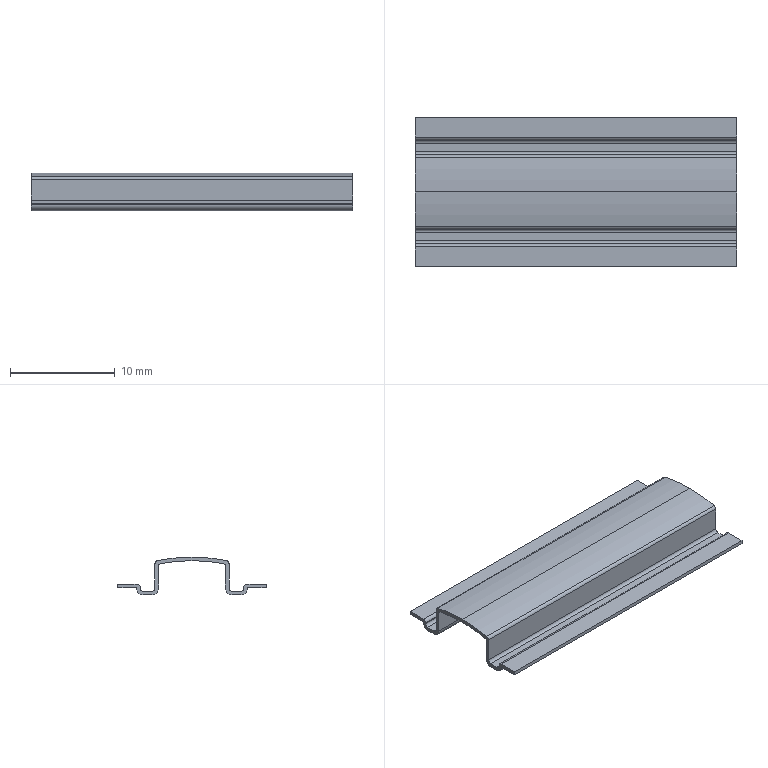Part | SolidWorks | features BaseBody 1 | 1 solid | 36 faces | box 30.643 x 14.143 x 3.615 mm | volume 220.482 mm3 | plane 20 | cylinder 16 | commonest cylinder face diameters 0.589 x8 1.296 x4 31.114 x2 31.821 x2
STEP:
#1=CARTESIAN_POINT('',(-15.321,5.304,12.964));
#2=VERTEX_POINT('',#1);
#3=CARTESIAN_POINT('',(-15.321,7.071,12.964));
#4=VERTEX_POINT('',#3);
#5=CARTESIAN_POINT('',(-15.321,5.245,12.964));
#6=DIRECTION('',(0.,1.,0.));
#7=VECTOR('',#6,1000.);
#8=LINE('',#5,#7);
#9=EDGE_CURVE('',#2,#4,#8,.T.);
#10=ORIENTED_EDGE('',*,*,#9,.F.);
#11=CARTESIAN_POINT('',(-15.321,5.304,12.944));
#12=VERTEX_POINT('',#11);
#13=CARTESIAN_POINT('',(-15.321,5.304,12.944));
#14=DIRECTION('',(0.,0.,1.));
#15=VECTOR('',#14,1000.);
#16=LINE('',#13,#15);
#17=EDGE_CURVE('',#12,#2,#16,.T.);
#18=ORIENTED_EDGE('',*,*,#17,.F.);
#19=CARTESIAN_POINT('',(-15.321,4.655,12.296));
#20=VERTEX_POINT('',#19);
#21=CARTESIAN_POINT('',(-15.321,4.655,12.944));
#22=DIRECTION('',(1.,0.,0.));
#23=DIRECTION('',(0.,0.,-1.));
#24=AXIS2_PLACEMENT_3D('',#21,#22,#23);
#25=CIRCLE('',#24,0.6482);
#26=EDGE_CURVE('',#20,#12,#25,.T.);
#27=ORIENTED_EDGE('',*,*,#26,.F.);
#28=CARTESIAN_POINT('',(-15.321,3.83,12.296));
#29=VERTEX_POINT('',#28);
#30=CARTESIAN_POINT('',(-15.321,3.83,12.296));
#31=DIRECTION('',(0.,1.,0.));
#32=VECTOR('',#31,1000.);
#33=LINE('',#30,#32);
#34=EDGE_CURVE('',#29,#20,#33,.T.);
#35=ORIENTED_EDGE('',*,*,#34,.F.);
#36=CARTESIAN_POINT('',(-15.321,3.182,12.944));
#37=VERTEX_POINT('',#36);
#38=CARTESIAN_POINT('',(-15.321,3.83,12.944));
#39=DIRECTION('',(1.,0.,0.));
#40=DIRECTION('',(0.,0.,-1.));
#41=AXIS2_PLACEMENT_3D('',#38,#39,#40);
#42=CIRCLE('',#41,0.6482);
#43=EDGE_CURVE('',#37,#29,#42,.T.);
#44=ORIENTED_EDGE('',*,*,#43,.F.);
#45=CARTESIAN_POINT('',(-15.321,3.182,15.228));
#46=VERTEX_POINT('',#45);
#47=CARTESIAN_POINT('',(-15.321,3.182,15.276));
#48=DIRECTION('',(0.,0.,-1.));
#49=VECTOR('',#48,1000.);
#50=LINE('',#47,#49);
#51=EDGE_CURVE('',#46,#37,#50,.T.);
#52=ORIENTED_EDGE('',*,*,#51,.F.);
#53=CARTESIAN_POINT('',(-15.321,0.,15.557));
#54=VERTEX_POINT('',#53);
#55=CARTESIAN_POINT('',(-15.321,0.,0.));
#56=DIRECTION('',(-1.,0.,0.));
#57=DIRECTION('',(0.,0.,-1.));
#58=AXIS2_PLACEMENT_3D('',#55,#56,#57);
#59=CIRCLE('',#58,15.557);
#60=EDGE_CURVE('',#54,#46,#59,.T.);
#61=ORIENTED_EDGE('',*,*,#60,.F.);
#62=CARTESIAN_POINT('',(-15.321,-3.182,15.228));
#63=VERTEX_POINT('',#62);
#64=CARTESIAN_POINT('',(-15.321,0.,0.));
#65=DIRECTION('',(-1.,0.,0.));
#66=DIRECTION('',(0.,0.,-1.));
#67=AXIS2_PLACEMENT_3D('',#64,#65,#66);
#68=CIRCLE('',#67,15.557);
#69=EDGE_CURVE('',#63,#54,#68,.T.);
#70=ORIENTED_EDGE('',*,*,#69,.F.);
#71=CARTESIAN_POINT('',(-15.321,-3.182,12.944));
#72=VERTEX_POINT('',#71);
#73=CARTESIAN_POINT('',(-15.321,-3.182,15.276));
#74=DIRECTION('',(0.,0.,1.));
#75=VECTOR('',#74,1000.);
#76=LINE('',#73,#75);
#77=EDGE_CURVE('',#72,#63,#76,.T.);
#78=ORIENTED_EDGE('',*,*,#77,.F.);
#79=CARTESIAN_POINT('',(-15.321,-3.83,12.296));
#80=VERTEX_POINT('',#79);
#81=CARTESIAN_POINT('',(-15.321,-3.83,12.944));
#82=DIRECTION('',(1.,0.,0.));
#83=DIRECTION('',(0.,0.,-1.));
#84=AXIS2_PLACEMENT_3D('',#81,#82,#83);
#85=CIRCLE('',#84,0.6482);
#86=EDGE_CURVE('',#80,#72,#85,.T.);
#87=ORIENTED_EDGE('',*,*,#86,.F.);
#88=CARTESIAN_POINT('',(-15.321,-4.655,12.296));
#89=VERTEX_POINT('',#88);
#90=CARTESIAN_POINT('',(-15.321,-3.83,12.296));
#91=DIRECTION('',(0.,1.,0.));
#92=VECTOR('',#91,1000.);
#93=LINE('',#90,#92);
#94=EDGE_CURVE('',#89,#80,#93,.T.);
#95=ORIENTED_EDGE('',*,*,#94,.F.);
#96=CARTESIAN_POINT('',(-15.321,-5.304,12.944));
#97=VERTEX_POINT('',#96);
#98=CARTESIAN_POINT('',(-15.321,-4.655,12.944));
#99=DIRECTION('',(1.,0.,0.));
#100=DIRECTION('',(0.,0.,-1.));
#101=AXIS2_PLACEMENT_3D('',#98,#99,#100);
#102=CIRCLE('',#101,0.6482);
#103=EDGE_CURVE('',#97,#89,#102,.T.);
#104=ORIENTED_EDGE('',*,*,#103,.F.);
#105=CARTESIAN_POINT('',(-15.321,-5.304,12.964));
#106=VERTEX_POINT('',#105);
#107=CARTESIAN_POINT('',(-15.321,-5.304,12.944));
#108=DIRECTION('',(0.,0.,-1.));
#109=VECTOR('',#108,1000.);
#110=LINE('',#107,#109);
#111=EDGE_CURVE('',#106,#97,#110,.T.);
#112=ORIENTED_EDGE('',*,*,#111,.F.);
#113=CARTESIAN_POINT('',(-15.321,-7.071,12.964));
#114=VERTEX_POINT('',#113);
#115=CARTESIAN_POINT('',(-15.321,-5.245,12.964));
#116=DIRECTION('',(0.,1.,0.));
#117=VECTOR('',#116,1000.);
#118=LINE('',#115,#117);
#119=EDGE_CURVE('',#114,#106,#118,.T.);
#120=ORIENTED_EDGE('',*,*,#119,.F.);
#121=CARTESIAN_POINT('',(-15.321,-7.071,13.318));
#122=VERTEX_POINT('',#121);
#123=CARTESIAN_POINT('',(-15.321,-7.071,12.964));
#124=DIRECTION('',(0.,0.,1.));
#125=VECTOR('',#124,1000.);
#126=LINE('',#123,#125);
#127=EDGE_CURVE('',#114,#122,#126,.T.);
#128=ORIENTED_EDGE('',*,*,#127,.T.);
#129=CARTESIAN_POINT('',(-15.321,-5.245,13.318));
#130=VERTEX_POINT('',#129);
#131=CARTESIAN_POINT('',(-15.321,-5.245,13.318));
#132=DIRECTION('',(0.,1.,0.));
#133=VECTOR('',#132,1000.);
#134=LINE('',#131,#133);
#135=EDGE_CURVE('',#122,#130,#134,.T.);
#136=ORIENTED_EDGE('',*,*,#135,.T.);
#137=CARTESIAN_POINT('',(-15.321,-4.95,13.023));
#138=VERTEX_POINT('',#137);
#139=CARTESIAN_POINT('',(-15.321,-5.245,13.023));
#140=DIRECTION('',(-1.,0.,0.));
#141=DIRECTION('',(0.,0.,1.));
#142=AXIS2_PLACEMENT_3D('',#139,#140,#141);
#143=CIRCLE('',#142,0.2946);
#144=EDGE_CURVE('',#130,#138,#143,.T.);
#145=ORIENTED_EDGE('',*,*,#144,.T.);
#146=CARTESIAN_POINT('',(-15.321,-4.95,12.944));
#147=VERTEX_POINT('',#146);
#148=CARTESIAN_POINT('',(-15.321,-4.95,12.944));
#149=DIRECTION('',(0.,0.,-1.));
#150=VECTOR('',#149,1000.);
#151=LINE('',#148,#150);
#152=EDGE_CURVE('',#138,#147,#151,.T.);
#153=ORIENTED_EDGE('',*,*,#152,.T.);
#154=CARTESIAN_POINT('',(-15.321,-4.655,12.65));
#155=VERTEX_POINT('',#154);
#156=CARTESIAN_POINT('',(-15.321,-4.655,12.944));
#157=DIRECTION('',(1.,0.,0.));
#158=DIRECTION('',(0.,0.,-1.));
#159=AXIS2_PLACEMENT_3D('',#156,#157,#158);
#160=CIRCLE('',#159,0.2946);
#161=EDGE_CURVE('',#147,#155,#160,.T.);
#162=ORIENTED_EDGE('',*,*,#161,.T.);
#163=CARTESIAN_POINT('',(-15.321,-3.83,12.65));
#164=VERTEX_POINT('',#163);
#165=CARTESIAN_POINT('',(-15.321,-3.83,12.65));
#166=DIRECTION('',(0.,1.,0.));
#167=VECTOR('',#166,1000.);
#168=LINE('',#165,#167);
#169=EDGE_CURVE('',#155,#164,#168,.T.);
#170=ORIENTED_EDGE('',*,*,#169,.T.);
#171=CARTESIAN_POINT('',(-15.321,-3.536,12.944));
#172=VERTEX_POINT('',#171);
#173=CARTESIAN_POINT('',(-15.321,-3.83,12.944));
#174=DIRECTION('',(1.,0.,0.));
#175=DIRECTION('',(0.,0.,-1.));
#176=AXIS2_PLACEMENT_3D('',#173,#174,#175);
#177=CIRCLE('',#176,0.2946);
#178=EDGE_CURVE('',#164,#172,#177,.T.);
#179=ORIENTED_EDGE('',*,*,#178,.T.);
#180=CARTESIAN_POINT('',(-15.321,-3.536,15.276));
#181=VERTEX_POINT('',#180);
#182=CARTESIAN_POINT('',(-15.321,-3.536,15.276));
#183=DIRECTION('',(0.,0.,1.));
#184=VECTOR('',#183,1000.);
#185=LINE('',#182,#184);
#186=EDGE_CURVE('',#172,#181,#185,.T.);
#187=ORIENTED_EDGE('',*,*,#186,.T.);
#188=CARTESIAN_POINT('',(-15.321,-3.302,15.564));
#189=VERTEX_POINT('',#188);
#190=CARTESIAN_POINT('',(-15.321,-3.241,15.276));
#191=DIRECTION('',(-1.,0.,0.));
#192=DIRECTION('',(0.,0.,1.));
#193=AXIS2_PLACEMENT_3D('',#190,#191,#192);
#194=CIRCLE('',#193,0.2946);
#195=EDGE_CURVE('',#181,#189,#194,.T.);
#196=ORIENTED_EDGE('',*,*,#195,.T.);
#197=CARTESIAN_POINT('',(-15.321,0.,15.911));
#198=VERTEX_POINT('',#197);
#199=CARTESIAN_POINT('',(-15.321,0.,0.));
#200=DIRECTION('',(-1.,0.,0.));
#201=DIRECTION('',(0.,0.,-1.));
#202=AXIS2_PLACEMENT_3D('',#199,#200,#201);
#203=CIRCLE('',#202,15.911);
#204=EDGE_CURVE('',#189,#198,#203,.T.);
#205=ORIENTED_EDGE('',*,*,#204,.T.);
#206=CARTESIAN_POINT('',(-15.321,3.302,15.564));
#207=VERTEX_POINT('',#206);
#208=CARTESIAN_POINT('',(-15.321,0.,0.));
#209=DIRECTION('',(-1.,0.,0.));
#210=DIRECTION('',(0.,0.,-1.));
#211=AXIS2_PLACEMENT_3D('',#208,#209,#210);
#212=CIRCLE('',#211,15.911);
#213=EDGE_CURVE('',#198,#207,#212,.T.);
#214=ORIENTED_EDGE('',*,*,#213,.T.);
#215=CARTESIAN_POINT('',(-15.321,3.536,15.276));
#216=VERTEX_POINT('',#215);
#217=CARTESIAN_POINT('',(-15.321,3.241,15.276));
#218=DIRECTION('',(-1.,0.,0.));
#219=DIRECTION('',(0.,0.,1.));
#220=AXIS2_PLACEMENT_3D('',#217,#218,#219);
#221=CIRCLE('',#220,0.2946);
#222=EDGE_CURVE('',#207,#216,#221,.T.);
#223=ORIENTED_EDGE('',*,*,#222,.T.);
#224=CARTESIAN_POINT('',(-15.321,3.536,12.944));
#225=VERTEX_POINT('',#224);
#226=CARTESIAN_POINT('',(-15.321,3.536,15.276));
#227=DIRECTION('',(0.,0.,-1.));
#228=VECTOR('',#227,1000.);
#229=LINE('',#226,#228);
#230=EDGE_CURVE('',#216,#225,#229,.T.);
#231=ORIENTED_EDGE('',*,*,#230,.T.);
#232=CARTESIAN_POINT('',(-15.321,3.83,12.65));
#233=VERTEX_POINT('',#232);
#234=CARTESIAN_POINT('',(-15.321,3.83,12.944));
#235=DIRECTION('',(1.,0.,0.));
#236=DIRECTION('',(0.,0.,-1.));
#237=AXIS2_PLACEMENT_3D('',#234,#235,#236);
#238=CIRCLE('',#237,0.2946);
#239=EDGE_CURVE('',#225,#233,#238,.T.);
#240=ORIENTED_EDGE('',*,*,#239,.T.);
#241=CARTESIAN_POINT('',(-15.321,4.655,12.65));
#242=VERTEX_POINT('',#241);
#243=CARTESIAN_POINT('',(-15.321,3.83,12.65));
#244=DIRECTION('',(0.,1.,0.));
#245=VECTOR('',#244,1000.);
#246=LINE('',#243,#245);
#247=EDGE_CURVE('',#233,#242,#246,.T.);
#248=ORIENTED_EDGE('',*,*,#247,.T.);
#249=CARTESIAN_POINT('',(-15.321,4.95,12.944));
#250=VERTEX_POINT('',#249);
#251=CARTESIAN_POINT('',(-15.321,4.655,12.944));
#252=DIRECTION('',(1.,0.,0.));
#253=DIRECTION('',(0.,0.,-1.));
#254=AXIS2_PLACEMENT_3D('',#251,#252,#253);
#255=CIRCLE('',#254,0.2946);
#256=EDGE_CURVE('',#242,#250,#255,.T.);
#257=ORIENTED_EDGE('',*,*,#256,.T.);
#258=CARTESIAN_POINT('',(-15.321,4.95,13.023));
#259=VERTEX_POINT('',#258);
#260=CARTESIAN_POINT('',(-15.321,4.95,12.944));
#261=DIRECTION('',(0.,0.,1.));
#262=VECTOR('',#261,1000.);
#263=LINE('',#260,#262);
#264=EDGE_CURVE('',#250,#259,#263,.T.);
#265=ORIENTED_EDGE('',*,*,#264,.T.);
#266=CARTESIAN_POINT('',(-15.321,5.245,13.318));
#267=VERTEX_POINT('',#266);
#268=CARTESIAN_POINT('',(-15.321,5.245,13.023));
#269=DIRECTION('',(-1.,0.,0.));
#270=DIRECTION('',(0.,0.,1.));
#271=AXIS2_PLACEMENT_3D('',#268,#269,#270);
#272=CIRCLE('',#271,0.2946);
#273=EDGE_CURVE('',#259,#267,#272,.T.);
#274=ORIENTED_EDGE('',*,*,#273,.T.);
#275=CARTESIAN_POINT('',(-15.321,7.071,13.318));
#276=VERTEX_POINT('',#275);
#277=CARTESIAN_POINT('',(-15.321,5.245,13.318));
#278=DIRECTION('',(0.,1.,0.));
#279=VECTOR('',#278,1000.);
#280=LINE('',#277,#279);
#281=EDGE_CURVE('',#267,#276,#280,.T.);
#282=ORIENTED_EDGE('',*,*,#281,.T.);
#283=CARTESIAN_POINT('',(-15.321,7.071,13.318));
#284=DIRECTION('',(0.,0.,-1.));
#285=VECTOR('',#284,1000.);
#286=LINE('',#283,#285);
#287=EDGE_CURVE('',#276,#4,#286,.T.);
#288=ORIENTED_EDGE('',*,*,#287,.T.);
#289=EDGE_LOOP('',(#10,#18,#27,#35,#44,#52,#61,#70,#78,#87,#95,#104,#112,#120,#128,#136,#145,#153,#162,#170,#179,#187,#196,#205,#214,#223,#231,#240,#248,#257,#265,#274,#282,#288));
#290=FACE_OUTER_BOUND('',#289,.T.);
#291=CARTESIAN_POINT('',(-15.321,5.245,13.023));
#292=DIRECTION('',(-1.,0.,0.));
#293=DIRECTION('',(0.,0.,1.));
#294=AXIS2_PLACEMENT_3D('',#291,#292,#293);
#295=PLANE('',#294);
#296=ADVANCED_FACE('',(#290),#295,.T.);
#297=CARTESIAN_POINT('',(15.321,5.304,12.964));
#298=VERTEX_POINT('',#297);
#299=CARTESIAN_POINT('',(15.321,7.071,12.964));
#300=VERTEX_POINT('',#299);
#301=CARTESIAN_POINT('',(15.321,5.245,12.964));
#302=DIRECTION('',(0.,1.,0.));
#303=VECTOR('',#302,1000.);
#304=LINE('',#301,#303);
#305=EDGE_CURVE('',#298,#300,#304,.T.);
#306=ORIENTED_EDGE('',*,*,#305,.T.);
#307=CARTESIAN_POINT('',(15.321,7.071,13.318));
#308=VERTEX_POINT('',#307);
#309=CARTESIAN_POINT('',(15.321,7.071,13.318));
#310=DIRECTION('',(0.,0.,-1.));
#311=VECTOR('',#310,1000.);
#312=LINE('',#309,#311);
#313=EDGE_CURVE('',#308,#300,#312,.T.);
#314=ORIENTED_EDGE('',*,*,#313,.F.);
#315=CARTESIAN_POINT('',(15.321,5.245,13.318));
#316=VERTEX_POINT('',#315);
#317=CARTESIAN_POINT('',(15.321,5.245,13.318));
#318=DIRECTION('',(0.,1.,0.));
#319=VECTOR('',#318,1000.);
#320=LINE('',#317,#319);
#321=EDGE_CURVE('',#316,#308,#320,.T.);
#322=ORIENTED_EDGE('',*,*,#321,.F.);
#323=CARTESIAN_POINT('',(15.321,4.95,13.023));
#324=VERTEX_POINT('',#323);
#325=CARTESIAN_POINT('',(15.321,5.245,13.023));
#326=DIRECTION('',(-1.,0.,0.));
#327=DIRECTION('',(0.,0.,1.));
#328=AXIS2_PLACEMENT_3D('',#325,#326,#327);
#329=CIRCLE('',#328,0.2946);
#330=EDGE_CURVE('',#324,#316,#329,.T.);
#331=ORIENTED_EDGE('',*,*,#330,.F.);
#332=CARTESIAN_POINT('',(15.321,4.95,12.944));
#333=VERTEX_POINT('',#332);
#334=CARTESIAN_POINT('',(15.321,4.95,12.944));
#335=DIRECTION('',(0.,0.,1.));
#336=VECTOR('',#335,1000.);
#337=LINE('',#334,#336);
#338=EDGE_CURVE('',#333,#324,#337,.T.);
#339=ORIENTED_EDGE('',*,*,#338,.F.);
#340=CARTESIAN_POINT('',(15.321,4.655,12.65));
#341=VERTEX_POINT('',#340);
#342=CARTESIAN_POINT('',(15.321,4.655,12.944));
#343=DIRECTION('',(1.,0.,0.));
#344=DIRECTION('',(0.,0.,-1.));
#345=AXIS2_PLACEMENT_3D('',#342,#343,#344);
#346=CIRCLE('',#345,0.2946);
#347=EDGE_CURVE('',#341,#333,#346,.T.);
#348=ORIENTED_EDGE('',*,*,#347,.F.);
#349=CARTESIAN_POINT('',(15.321,3.83,12.65));
#350=VERTEX_POINT('',#349);
#351=CARTESIAN_POINT('',(15.321,3.83,12.65));
#352=DIRECTION('',(0.,1.,0.));
#353=VECTOR('',#352,1000.);
#354=LINE('',#351,#353);
#355=EDGE_CURVE('',#350,#341,#354,.T.);
#356=ORIENTED_EDGE('',*,*,#355,.F.);
#357=CARTESIAN_POINT('',(15.321,3.536,12.944));
#358=VERTEX_POINT('',#357);
#359=CARTESIAN_POINT('',(15.321,3.83,12.944));
#360=DIRECTION('',(1.,0.,0.));
#361=DIRECTION('',(0.,0.,-1.));
#362=AXIS2_PLACEMENT_3D('',#359,#360,#361);
#363=CIRCLE('',#362,0.2946);
#364=EDGE_CURVE('',#358,#350,#363,.T.);
#365=ORIENTED_EDGE('',*,*,#364,.F.);
#366=CARTESIAN_POINT('',(15.321,3.536,15.276));
#367=VERTEX_POINT('',#366);
#368=CARTESIAN_POINT('',(15.321,3.536,15.276));
#369=DIRECTION('',(0.,0.,-1.));
#370=VECTOR('',#369,1000.);
#371=LINE('',#368,#370);
#372=EDGE_CURVE('',#367,#358,#371,.T.);
#373=ORIENTED_EDGE('',*,*,#372,.F.);
#374=CARTESIAN_POINT('',(15.321,3.302,15.564));
#375=VERTEX_POINT('',#374);
#376=CARTESIAN_POINT('',(15.321,3.241,15.276));
#377=DIRECTION('',(-1.,0.,0.));
#378=DIRECTION('',(0.,0.,1.));
#379=AXIS2_PLACEMENT_3D('',#376,#377,#378);
#380=CIRCLE('',#379,0.2946);
#381=EDGE_CURVE('',#375,#367,#380,.T.);
#382=ORIENTED_EDGE('',*,*,#381,.F.);
#383=CARTESIAN_POINT('',(15.321,0.,15.911));
#384=VERTEX_POINT('',#383);
#385=CARTESIAN_POINT('',(15.321,0.,0.));
#386=DIRECTION('',(-1.,0.,0.));
#387=DIRECTION('',(0.,0.,-1.));
#388=AXIS2_PLACEMENT_3D('',#385,#386,#387);
#389=CIRCLE('',#388,15.911);
#390=EDGE_CURVE('',#384,#375,#389,.T.);
#391=ORIENTED_EDGE('',*,*,#390,.F.);
#392=CARTESIAN_POINT('',(15.321,-3.302,15.564));
#393=VERTEX_POINT('',#392);
#394=CARTESIAN_POINT('',(15.321,0.,0.));
#395=DIRECTION('',(-1.,0.,0.));
#396=DIRECTION('',(0.,0.,-1.));
#397=AXIS2_PLACEMENT_3D('',#394,#395,#396);
#398=CIRCLE('',#397,15.911);
#399=EDGE_CURVE('',#393,#384,#398,.T.);
#400=ORIENTED_EDGE('',*,*,#399,.F.);
#401=CARTESIAN_POINT('',(15.321,-3.536,15.276));
#402=VERTEX_POINT('',#401);
#403=CARTESIAN_POINT('',(15.321,-3.241,15.276));
#404=DIRECTION('',(-1.,0.,0.));
#405=DIRECTION('',(0.,0.,1.));
#406=AXIS2_PLACEMENT_3D('',#403,#404,#405);
#407=CIRCLE('',#406,0.2946);
#408=EDGE_CURVE('',#402,#393,#407,.T.);
#409=ORIENTED_EDGE('',*,*,#408,.F.);
#410=CARTESIAN_POINT('',(15.321,-3.536,12.944));
#411=VERTEX_POINT('',#410);
#412=CARTESIAN_POINT('',(15.321,-3.536,15.276));
#413=DIRECTION('',(0.,0.,1.));
#414=VECTOR('',#413,1000.);
#415=LINE('',#412,#414);
#416=EDGE_CURVE('',#411,#402,#415,.T.);
#417=ORIENTED_EDGE('',*,*,#416,.F.);
#418=CARTESIAN_POINT('',(15.321,-3.83,12.65));
#419=VERTEX_POINT('',#418);
#420=CARTESIAN_POINT('',(15.321,-3.83,12.944));
#421=DIRECTION('',(1.,0.,0.));
#422=DIRECTION('',(0.,0.,-1.));
#423=AXIS2_PLACEMENT_3D('',#420,#421,#422);
#424=CIRCLE('',#423,0.2946);
#425=EDGE_CURVE('',#419,#411,#424,.T.);
#426=ORIENTED_EDGE('',*,*,#425,.F.);
#427=CARTESIAN_POINT('',(15.321,-4.655,12.65));
#428=VERTEX_POINT('',#427);
#429=CARTESIAN_POINT('',(15.321,-3.83,12.65));
#430=DIRECTION('',(0.,1.,0.));
#431=VECTOR('',#430,1000.);
#432=LINE('',#429,#431);
#433=EDGE_CURVE('',#428,#419,#432,.T.);
#434=ORIENTED_EDGE('',*,*,#433,.F.);
#435=CARTESIAN_POINT('',(15.321,-4.95,12.944));
#436=VERTEX_POINT('',#435);
#437=CARTESIAN_POINT('',(15.321,-4.655,12.944));
#438=DIRECTION('',(1.,0.,0.));
#439=DIRECTION('',(0.,0.,-1.));
#440=AXIS2_PLACEMENT_3D('',#437,#438,#439);
#441=CIRCLE('',#440,0.2946);
#442=EDGE_CURVE('',#436,#428,#441,.T.);
#443=ORIENTED_EDGE('',*,*,#442,.F.);
#444=CARTESIAN_POINT('',(15.321,-4.95,13.023));
#445=VERTEX_POINT('',#444);
#446=CARTESIAN_POINT('',(15.321,-4.95,12.944));
#447=DIRECTION('',(0.,0.,-1.));
#448=VECTOR('',#447,1000.);
#449=LINE('',#446,#448);
#450=EDGE_CURVE('',#445,#436,#449,.T.);
#451=ORIENTED_EDGE('',*,*,#450,.F.);
#452=CARTESIAN_POINT('',(15.321,-5.245,13.318));
#453=VERTEX_POINT('',#452);
#454=CARTESIAN_POINT('',(15.321,-5.245,13.023));
#455=DIRECTION('',(-1.,0.,0.));
#456=DIRECTION('',(0.,0.,1.));
#457=AXIS2_PLACEMENT_3D('',#454,#455,#456);
#458=CIRCLE('',#457,0.2946);
#459=EDGE_CURVE('',#453,#445,#458,.T.);
#460=ORIENTED_EDGE('',*,*,#459,.F.);
#461=CARTESIAN_POINT('',(15.321,-7.071,13.318));
#462=VERTEX_POINT('',#461);
#463=CARTESIAN_POINT('',(15.321,-5.245,13.318));
#464=DIRECTION('',(0.,1.,0.));
#465=VECTOR('',#464,1000.);
#466=LINE('',#463,#465);
#467=EDGE_CURVE('',#462,#453,#466,.T.);
#468=ORIENTED_EDGE('',*,*,#467,.F.);
#469=CARTESIAN_POINT('',(15.321,-7.071,12.964));
#470=VERTEX_POINT('',#469);
#471=CARTESIAN_POINT('',(15.321,-7.071,12.964));
#472=DIRECTION('',(0.,0.,1.));
#473=VECTOR('',#472,1000.);
#474=LINE('',#471,#473);
#475=EDGE_CURVE('',#470,#462,#474,.T.);
#476=ORIENTED_EDGE('',*,*,#475,.F.);
#477=CARTESIAN_POINT('',(15.321,-5.304,12.964));
#478=VERTEX_POINT('',#477);
#479=CARTESIAN_POINT('',(15.321,-5.245,12.964));
#480=DIRECTION('',(0.,1.,0.));
#481=VECTOR('',#480,1000.);
#482=LINE('',#479,#481);
#483=EDGE_CURVE('',#470,#478,#482,.T.);
#484=ORIENTED_EDGE('',*,*,#483,.T.);
#485=CARTESIAN_POINT('',(15.321,-5.304,12.944));
#486=VERTEX_POINT('',#485);
#487=CARTESIAN_POINT('',(15.321,-5.304,12.944));
#488=DIRECTION('',(0.,0.,-1.));
#489=VECTOR('',#488,1000.);
#490=LINE('',#487,#489);
#491=EDGE_CURVE('',#478,#486,#490,.T.);
#492=ORIENTED_EDGE('',*,*,#491,.T.);
#493=CARTESIAN_POINT('',(15.321,-4.655,12.296));
#494=VERTEX_POINT('',#493);
#495=CARTESIAN_POINT('',(15.321,-4.655,12.944));
#496=DIRECTION('',(1.,0.,0.));
#497=DIRECTION('',(0.,0.,-1.));
#498=AXIS2_PLACEMENT_3D('',#495,#496,#497);
#499=CIRCLE('',#498,0.6482);
#500=EDGE_CURVE('',#486,#494,#499,.T.);
#501=ORIENTED_EDGE('',*,*,#500,.T.);
#502=CARTESIAN_POINT('',(15.321,-3.83,12.296));
#503=VERTEX_POINT('',#502);
#504=CARTESIAN_POINT('',(15.321,-3.83,12.296));
#505=DIRECTION('',(0.,1.,0.));
#506=VECTOR('',#505,1000.);
#507=LINE('',#504,#506);
#508=EDGE_CURVE('',#494,#503,#507,.T.);
#509=ORIENTED_EDGE('',*,*,#508,.T.);
#510=CARTESIAN_POINT('',(15.321,-3.182,12.944));
#511=VERTEX_POINT('',#510);
#512=CARTESIAN_POINT('',(15.321,-3.83,12.944));
#513=DIRECTION('',(1.,0.,0.));
#514=DIRECTION('',(0.,0.,-1.));
#515=AXIS2_PLACEMENT_3D('',#512,#513,#514);
#516=CIRCLE('',#515,0.6482);
#517=EDGE_CURVE('',#503,#511,#516,.T.);
#518=ORIENTED_EDGE('',*,*,#517,.T.);
#519=CARTESIAN_POINT('',(15.321,-3.182,15.228));
#520=VERTEX_POINT('',#519);
#521=CARTESIAN_POINT('',(15.321,-3.182,15.276));
#522=DIRECTION('',(0.,0.,1.));
#523=VECTOR('',#522,1000.);
#524=LINE('',#521,#523);
#525=EDGE_CURVE('',#511,#520,#524,.T.);
#526=ORIENTED_EDGE('',*,*,#525,.T.);
#527=CARTESIAN_POINT('',(15.321,0.,15.557));
#528=VERTEX_POINT('',#527);
#529=CARTESIAN_POINT('',(15.321,0.,0.));
#530=DIRECTION('',(-1.,0.,0.));
#531=DIRECTION('',(0.,0.,-1.));
#532=AXIS2_PLACEMENT_3D('',#529,#530,#531);
#533=CIRCLE('',#532,15.557);
#534=EDGE_CURVE('',#520,#528,#533,.T.);
#535=ORIENTED_EDGE('',*,*,#534,.T.);
#536=CARTESIAN_POINT('',(15.321,3.182,15.228));
#537=VERTEX_POINT('',#536);
#538=CARTESIAN_POINT('',(15.321,0.,0.));
#539=DIRECTION('',(-1.,0.,0.));
#540=DIRECTION('',(0.,0.,-1.));
#541=AXIS2_PLACEMENT_3D('',#538,#539,#540);
#542=CIRCLE('',#541,15.557);
#543=EDGE_CURVE('',#528,#537,#542,.T.);
#544=ORIENTED_EDGE('',*,*,#543,.T.);
#545=CARTESIAN_POINT('',(15.321,3.182,12.944));
#546=VERTEX_POINT('',#545);
#547=CARTESIAN_POINT('',(15.321,3.182,15.276));
#548=DIRECTION('',(0.,0.,-1.));
#549=VECTOR('',#548,1000.);
#550=LINE('',#547,#549);
#551=EDGE_CURVE('',#537,#546,#550,.T.);
#552=ORIENTED_EDGE('',*,*,#551,.T.);
#553=CARTESIAN_POINT('',(15.321,3.83,12.296));
#554=VERTEX_POINT('',#553);
#555=CARTESIAN_POINT('',(15.321,3.83,12.944));
#556=DIRECTION('',(1.,0.,0.));
#557=DIRECTION('',(0.,0.,-1.));
#558=AXIS2_PLACEMENT_3D('',#555,#556,#557);
#559=CIRCLE('',#558,0.6482);
#560=EDGE_CURVE('',#546,#554,#559,.T.);
#561=ORIENTED_EDGE('',*,*,#560,.T.);
#562=CARTESIAN_POINT('',(15.321,4.655,12.296));
#563=VERTEX_POINT('',#562);
#564=CARTESIAN_POINT('',(15.321,3.83,12.296));
#565=DIRECTION('',(0.,1.,0.));
#566=VECTOR('',#565,1000.);
#567=LINE('',#564,#566);
#568=EDGE_CURVE('',#554,#563,#567,.T.);
#569=ORIENTED_EDGE('',*,*,#568,.T.);
#570=CARTESIAN_POINT('',(15.321,5.304,12.944));
#571=VERTEX_POINT('',#570);
#572=CARTESIAN_POINT('',(15.321,4.655,12.944));
#573=DIRECTION('',(1.,0.,0.));
#574=DIRECTION('',(0.,0.,-1.));
#575=AXIS2_PLACEMENT_3D('',#572,#573,#574);
#576=CIRCLE('',#575,0.6482);
#577=EDGE_CURVE('',#563,#571,#576,.T.);
#578=ORIENTED_EDGE('',*,*,#577,.T.);
#579=CARTESIAN_POINT('',(15.321,5.304,12.944));
#580=DIRECTION('',(0.,0.,1.));
#581=VECTOR('',#580,1000.);
#582=LINE('',#579,#581);
#583=EDGE_CURVE('',#571,#298,#582,.T.);
#584=ORIENTED_EDGE('',*,*,#583,.T.);
#585=EDGE_LOOP('',(#306,#314,#322,#331,#339,#348,#356,#365,#373,#382,#391,#400,#409,#417,#426,#434,#443,#451,#460,#468,#476,#484,#492,#501,#509,#518,#526,#535,#544,#552,#561,#569,#578,#584));
#586=FACE_OUTER_BOUND('',#585,.T.);
#587=CARTESIAN_POINT('',(15.321,5.245,13.023));
#588=DIRECTION('',(-1.,0.,0.));
#589=DIRECTION('',(0.,0.,1.));
#590=AXIS2_PLACEMENT_3D('',#587,#588,#589);
#591=PLANE('',#590);
#592=ADVANCED_FACE('',(#586),#591,.F.);
#593=ORIENTED_EDGE('',*,*,#17,.T.);
#594=CARTESIAN_POINT('',(15.321,5.304,12.964));
#595=DIRECTION('',(-1.,0.,0.));
#596=VECTOR('',#595,1000.);
#597=LINE('',#594,#596);
#598=EDGE_CURVE('',#298,#2,#597,.T.);
#599=ORIENTED_EDGE('',*,*,#598,.F.);
#600=ORIENTED_EDGE('',*,*,#583,.F.);
#601=CARTESIAN_POINT('',(15.321,5.304,12.944));
#602=DIRECTION('',(-1.,0.,0.));
#603=VECTOR('',#602,1000.);
#604=LINE('',#601,#603);
#605=EDGE_CURVE('',#571,#12,#604,.T.);
#606=ORIENTED_EDGE('',*,*,#605,.T.);
#607=EDGE_LOOP('',(#593,#599,#600,#606));
#608=FACE_OUTER_BOUND('',#607,.T.);
#609=CARTESIAN_POINT('',(15.321,5.304,12.944));
#610=DIRECTION('',(0.,-1.,0.));
#611=DIRECTION('',(0.,0.,-1.));
#612=AXIS2_PLACEMENT_3D('',#609,#610,#611);
#613=PLANE('',#612);
#614=ADVANCED_FACE('',(#608),#613,.F.);
#615=ORIENTED_EDGE('',*,*,#26,.T.);
#616=ORIENTED_EDGE('',*,*,#605,.F.);
#617=ORIENTED_EDGE('',*,*,#577,.F.);
#618=CARTESIAN_POINT('',(15.321,4.655,12.296));
#619=DIRECTION('',(-1.,0.,0.));
#620=VECTOR('',#619,1000.);
#621=LINE('',#618,#620);
#622=EDGE_CURVE('',#563,#20,#621,.T.);
#623=ORIENTED_EDGE('',*,*,#622,.T.);
#624=EDGE_LOOP('',(#615,#616,#617,#623));
#625=FACE_OUTER_BOUND('',#624,.T.);
#626=CARTESIAN_POINT('',(15.321,4.655,12.944));
#627=DIRECTION('',(-1.,0.,0.));
#628=DIRECTION('',(0.,0.,1.));
#629=AXIS2_PLACEMENT_3D('',#626,#627,#628);
#630=CYLINDRICAL_SURFACE('',#629,0.6482);
#631=ADVANCED_FACE('',(#625),#630,.T.);
#632=ORIENTED_EDGE('',*,*,#34,.T.);
#633=ORIENTED_EDGE('',*,*,#622,.F.);
#634=ORIENTED_EDGE('',*,*,#568,.F.);
#635=CARTESIAN_POINT('',(15.321,3.83,12.296));
#636=DIRECTION('',(-1.,0.,0.));
#637=VECTOR('',#636,1000.);
#638=LINE('',#635,#637);
#639=EDGE_CURVE('',#554,#29,#638,.T.);
#640=ORIENTED_EDGE('',*,*,#639,.T.);
#641=EDGE_LOOP('',(#632,#633,#634,#640));
#642=FACE_OUTER_BOUND('',#641,.T.);
#643=CARTESIAN_POINT('',(15.321,3.83,12.296));
#644=DIRECTION('',(0.,0.,1.));
#645=DIRECTION('',(1.,0.,0.));
#646=AXIS2_PLACEMENT_3D('',#643,#644,#645);
#647=PLANE('',#646);
#648=ADVANCED_FACE('',(#642),#647,.F.);
#649=ORIENTED_EDGE('',*,*,#43,.T.);
#650=ORIENTED_EDGE('',*,*,#639,.F.);
#651=ORIENTED_EDGE('',*,*,#560,.F.);
#652=CARTESIAN_POINT('',(15.321,3.182,12.944));
#653=DIRECTION('',(-1.,0.,0.));
#654=VECTOR('',#653,1000.);
#655=LINE('',#652,#654);
#656=EDGE_CURVE('',#546,#37,#655,.T.);
#657=ORIENTED_EDGE('',*,*,#656,.T.);
#658=EDGE_LOOP('',(#649,#650,#651,#657));
#659=FACE_OUTER_BOUND('',#658,.T.);
#660=CARTESIAN_POINT('',(15.321,3.83,12.944));
#661=DIRECTION('',(-1.,0.,0.));
#662=DIRECTION('',(0.,0.,1.));
#663=AXIS2_PLACEMENT_3D('',#660,#661,#662);
#664=CYLINDRICAL_SURFACE('',#663,0.6482);
#665=ADVANCED_FACE('',(#659),#664,.T.);
#666=ORIENTED_EDGE('',*,*,#51,.T.);
#667=ORIENTED_EDGE('',*,*,#656,.F.);
#668=ORIENTED_EDGE('',*,*,#551,.F.);
#669=CARTESIAN_POINT('',(15.321,3.182,15.228));
#670=DIRECTION('',(-1.,0.,0.));
#671=VECTOR('',#670,1000.);
#672=LINE('',#669,#671);
#673=EDGE_CURVE('',#537,#46,#672,.T.);
#674=ORIENTED_EDGE('',*,*,#673,.T.);
#675=EDGE_LOOP('',(#666,#667,#668,#674));
#676=FACE_OUTER_BOUND('',#675,.T.);
#677=CARTESIAN_POINT('',(15.321,3.182,15.276));
#678=DIRECTION('',(0.,1.,0.));
#679=DIRECTION('',(1.,0.,0.));
#680=AXIS2_PLACEMENT_3D('',#677,#678,#679);
#681=PLANE('',#680);
#682=ADVANCED_FACE('',(#676),#681,.F.);
#683=CARTESIAN_POINT('',(15.321,0.,15.557));
#684=DIRECTION('',(-1.,0.,0.));
#685=VECTOR('',#684,1000.);
#686=LINE('',#683,#685);
#687=EDGE_CURVE('',#528,#54,#686,.T.);
#688=ORIENTED_EDGE('',*,*,#687,.F.);
#689=ORIENTED_EDGE('',*,*,#534,.F.);
#690=CARTESIAN_POINT('',(15.321,-3.182,15.228));
#691=DIRECTION('',(-1.,0.,0.));
#692=VECTOR('',#691,1000.);
#693=LINE('',#690,#692);
#694=EDGE_CURVE('',#520,#63,#693,.T.);
#695=ORIENTED_EDGE('',*,*,#694,.T.);
#696=ORIENTED_EDGE('',*,*,#69,.T.);
#697=EDGE_LOOP('',(#688,#689,#695,#696));
#698=FACE_OUTER_BOUND('',#697,.T.);
#699=CARTESIAN_POINT('',(15.321,0.,0.));
#700=DIRECTION('',(-1.,0.,0.));
#701=DIRECTION('',(0.,0.,1.));
#702=AXIS2_PLACEMENT_3D('',#699,#700,#701);
#703=CYLINDRICAL_SURFACE('',#702,15.557);
#704=ADVANCED_FACE('',(#698),#703,.F.);
#705=ORIENTED_EDGE('',*,*,#77,.T.);
#706=ORIENTED_EDGE('',*,*,#694,.F.);
#707=ORIENTED_EDGE('',*,*,#525,.F.);
#708=CARTESIAN_POINT('',(15.321,-3.182,12.944));
#709=DIRECTION('',(-1.,0.,0.));
#710=VECTOR('',#709,1000.);
#711=LINE('',#708,#710);
#712=EDGE_CURVE('',#511,#72,#711,.T.);
#713=ORIENTED_EDGE('',*,*,#712,.T.);
#714=EDGE_LOOP('',(#705,#706,#707,#713));
#715=FACE_OUTER_BOUND('',#714,.T.);
#716=CARTESIAN_POINT('',(15.321,-3.182,15.276));
#717=DIRECTION('',(0.,-1.,0.));
#718=DIRECTION('',(0.,0.,-1.));
#719=AXIS2_PLACEMENT_3D('',#716,#717,#718);
#720=PLANE('',#719);
#721=ADVANCED_FACE('',(#715),#720,.F.);
#722=ORIENTED_EDGE('',*,*,#86,.T.);
#723=ORIENTED_EDGE('',*,*,#712,.F.);
#724=ORIENTED_EDGE('',*,*,#517,.F.);
#725=CARTESIAN_POINT('',(15.321,-3.83,12.296));
#726=DIRECTION('',(-1.,0.,0.));
#727=VECTOR('',#726,1000.);
#728=LINE('',#725,#727);
#729=EDGE_CURVE('',#503,#80,#728,.T.);
#730=ORIENTED_EDGE('',*,*,#729,.T.);
#731=EDGE_LOOP('',(#722,#723,#724,#730));
#732=FACE_OUTER_BOUND('',#731,.T.);
#733=CARTESIAN_POINT('',(15.321,-3.83,12.944));
#734=DIRECTION('',(-1.,0.,0.));
#735=DIRECTION('',(0.,0.,1.));
#736=AXIS2_PLACEMENT_3D('',#733,#734,#735);
#737=CYLINDRICAL_SURFACE('',#736,0.6482);
#738=ADVANCED_FACE('',(#732),#737,.T.);
#739=ORIENTED_EDGE('',*,*,#94,.T.);
#740=ORIENTED_EDGE('',*,*,#729,.F.);
#741=ORIENTED_EDGE('',*,*,#508,.F.);
#742=CARTESIAN_POINT('',(15.321,-4.655,12.296));
#743=DIRECTION('',(-1.,0.,0.));
#744=VECTOR('',#743,1000.);
#745=LINE('',#742,#744);
#746=EDGE_CURVE('',#494,#89,#745,.T.);
#747=ORIENTED_EDGE('',*,*,#746,.T.);
#748=EDGE_LOOP('',(#739,#740,#741,#747));
#749=FACE_OUTER_BOUND('',#748,.T.);
#750=CARTESIAN_POINT('',(15.321,-3.83,12.296));
#751=DIRECTION('',(0.,0.,1.));
#752=DIRECTION('',(1.,0.,0.));
#753=AXIS2_PLACEMENT_3D('',#750,#751,#752);
#754=PLANE('',#753);
#755=ADVANCED_FACE('',(#749),#754,.F.);
#756=ORIENTED_EDGE('',*,*,#103,.T.);
#757=ORIENTED_EDGE('',*,*,#746,.F.);
#758=ORIENTED_EDGE('',*,*,#500,.F.);
#759=CARTESIAN_POINT('',(15.321,-5.304,12.944));
#760=DIRECTION('',(-1.,0.,0.));
#761=VECTOR('',#760,1000.);
#762=LINE('',#759,#761);
#763=EDGE_CURVE('',#486,#97,#762,.T.);
#764=ORIENTED_EDGE('',*,*,#763,.T.);
#765=EDGE_LOOP('',(#756,#757,#758,#764));
#766=FACE_OUTER_BOUND('',#765,.T.);
#767=CARTESIAN_POINT('',(15.321,-4.655,12.944));
#768=DIRECTION('',(-1.,0.,0.));
#769=DIRECTION('',(0.,0.,1.));
#770=AXIS2_PLACEMENT_3D('',#767,#768,#769);
#771=CYLINDRICAL_SURFACE('',#770,0.6482);
#772=ADVANCED_FACE('',(#766),#771,.T.);
#773=ORIENTED_EDGE('',*,*,#111,.T.);
#774=ORIENTED_EDGE('',*,*,#763,.F.);
#775=ORIENTED_EDGE('',*,*,#491,.F.);
#776=CARTESIAN_POINT('',(15.321,-5.304,12.964));
#777=DIRECTION('',(-1.,0.,0.));
#778=VECTOR('',#777,1000.);
#779=LINE('',#776,#778);
#780=EDGE_CURVE('',#478,#106,#779,.T.);
#781=ORIENTED_EDGE('',*,*,#780,.T.);
#782=EDGE_LOOP('',(#773,#774,#775,#781));
#783=FACE_OUTER_BOUND('',#782,.T.);
#784=CARTESIAN_POINT('',(15.321,-5.304,12.944));
#785=DIRECTION('',(0.,1.,0.));
#786=DIRECTION('',(1.,0.,0.));
#787=AXIS2_PLACEMENT_3D('',#784,#785,#786);
#788=PLANE('',#787);
#789=ADVANCED_FACE('',(#783),#788,.F.);
#790=ORIENTED_EDGE('',*,*,#119,.T.);
#791=ORIENTED_EDGE('',*,*,#780,.F.);
#792=ORIENTED_EDGE('',*,*,#483,.F.);
#793=CARTESIAN_POINT('',(15.321,-7.071,12.964));
#794=DIRECTION('',(-1.,0.,0.));
#795=VECTOR('',#794,1000.);
#796=LINE('',#793,#795);
#797=EDGE_CURVE('',#470,#114,#796,.T.);
#798=ORIENTED_EDGE('',*,*,#797,.T.);
#799=EDGE_LOOP('',(#790,#791,#792,#798));
#800=FACE_OUTER_BOUND('',#799,.T.);
#801=CARTESIAN_POINT('',(15.321,-5.245,12.964));
#802=DIRECTION('',(0.,0.,1.));
#803=DIRECTION('',(1.,0.,0.));
#804=AXIS2_PLACEMENT_3D('',#801,#802,#803);
#805=PLANE('',#804);
#806=ADVANCED_FACE('',(#800),#805,.F.);
#807=ORIENTED_EDGE('',*,*,#127,.F.);
#808=ORIENTED_EDGE('',*,*,#797,.F.);
#809=ORIENTED_EDGE('',*,*,#475,.T.);
#810=CARTESIAN_POINT('',(15.321,-7.071,13.318));
#811=DIRECTION('',(-1.,0.,0.));
#812=VECTOR('',#811,1000.);
#813=LINE('',#810,#812);
#814=EDGE_CURVE('',#462,#122,#813,.T.);
#815=ORIENTED_EDGE('',*,*,#814,.T.);
#816=EDGE_LOOP('',(#807,#808,#809,#815));
#817=FACE_OUTER_BOUND('',#816,.T.);
#818=CARTESIAN_POINT('',(15.321,-7.071,12.964));
#819=DIRECTION('',(0.,-1.,0.));
#820=DIRECTION('',(0.,0.,-1.));
#821=AXIS2_PLACEMENT_3D('',#818,#819,#820);
#822=PLANE('',#821);
#823=ADVANCED_FACE('',(#817),#822,.T.);
#824=ORIENTED_EDGE('',*,*,#135,.F.);
#825=ORIENTED_EDGE('',*,*,#814,.F.);
#826=ORIENTED_EDGE('',*,*,#467,.T.);
#827=CARTESIAN_POINT('',(15.321,-5.245,13.318));
#828=DIRECTION('',(-1.,0.,0.));
#829=VECTOR('',#828,1000.);
#830=LINE('',#827,#829);
#831=EDGE_CURVE('',#453,#130,#830,.T.);
#832=ORIENTED_EDGE('',*,*,#831,.T.);
#833=EDGE_LOOP('',(#824,#825,#826,#832));
#834=FACE_OUTER_BOUND('',#833,.T.);
#835=CARTESIAN_POINT('',(15.321,-5.245,13.318));
#836=DIRECTION('',(0.,0.,1.));
#837=DIRECTION('',(1.,0.,0.));
#838=AXIS2_PLACEMENT_3D('',#835,#836,#837);
#839=PLANE('',#838);
#840=ADVANCED_FACE('',(#834),#839,.T.);
#841=ORIENTED_EDGE('',*,*,#144,.F.);
#842=ORIENTED_EDGE('',*,*,#831,.F.);
#843=ORIENTED_EDGE('',*,*,#459,.T.);
#844=CARTESIAN_POINT('',(15.321,-4.95,13.023));
#845=DIRECTION('',(-1.,0.,0.));
#846=VECTOR('',#845,1000.);
#847=LINE('',#844,#846);
#848=EDGE_CURVE('',#445,#138,#847,.T.);
#849=ORIENTED_EDGE('',*,*,#848,.T.);
#850=EDGE_LOOP('',(#841,#842,#843,#849));
#851=FACE_OUTER_BOUND('',#850,.T.);
#852=CARTESIAN_POINT('',(15.321,-5.245,13.023));
#853=DIRECTION('',(-1.,0.,0.));
#854=DIRECTION('',(0.,0.,1.));
#855=AXIS2_PLACEMENT_3D('',#852,#853,#854);
#856=CYLINDRICAL_SURFACE('',#855,0.2946);
#857=ADVANCED_FACE('',(#851),#856,.T.);
#858=ORIENTED_EDGE('',*,*,#152,.F.);
#859=ORIENTED_EDGE('',*,*,#848,.F.);
#860=ORIENTED_EDGE('',*,*,#450,.T.);
#861=CARTESIAN_POINT('',(15.321,-4.95,12.944));
#862=DIRECTION('',(-1.,0.,0.));
#863=VECTOR('',#862,1000.);
#864=LINE('',#861,#863);
#865=EDGE_CURVE('',#436,#147,#864,.T.);
#866=ORIENTED_EDGE('',*,*,#865,.T.);
#867=EDGE_LOOP('',(#858,#859,#860,#866));
#868=FACE_OUTER_BOUND('',#867,.T.);
#869=CARTESIAN_POINT('',(15.321,-4.95,12.944));
#870=DIRECTION('',(0.,1.,0.));
#871=DIRECTION('',(1.,0.,0.));
#872=AXIS2_PLACEMENT_3D('',#869,#870,#871);
#873=PLANE('',#872);
#874=ADVANCED_FACE('',(#868),#873,.T.);
#875=ORIENTED_EDGE('',*,*,#161,.F.);
#876=ORIENTED_EDGE('',*,*,#865,.F.);
#877=ORIENTED_EDGE('',*,*,#442,.T.);
#878=CARTESIAN_POINT('',(15.321,-4.655,12.65));
#879=DIRECTION('',(-1.,0.,0.));
#880=VECTOR('',#879,1000.);
#881=LINE('',#878,#880);
#882=EDGE_CURVE('',#428,#155,#881,.T.);
#883=ORIENTED_EDGE('',*,*,#882,.T.);
#884=EDGE_LOOP('',(#875,#876,#877,#883));
#885=FACE_OUTER_BOUND('',#884,.T.);
#886=CARTESIAN_POINT('',(15.321,-4.655,12.944));
#887=DIRECTION('',(-1.,0.,0.));
#888=DIRECTION('',(0.,0.,1.));
#889=AXIS2_PLACEMENT_3D('',#886,#887,#888);
#890=CYLINDRICAL_SURFACE('',#889,0.2946);
#891=ADVANCED_FACE('',(#885),#890,.F.);
#892=ORIENTED_EDGE('',*,*,#169,.F.);
#893=ORIENTED_EDGE('',*,*,#882,.F.);
#894=ORIENTED_EDGE('',*,*,#433,.T.);
#895=CARTESIAN_POINT('',(15.321,-3.83,12.65));
#896=DIRECTION('',(-1.,0.,0.));
#897=VECTOR('',#896,1000.);
#898=LINE('',#895,#897);
#899=EDGE_CURVE('',#419,#164,#898,.T.);
#900=ORIENTED_EDGE('',*,*,#899,.T.);
#901=EDGE_LOOP('',(#892,#893,#894,#900));
#902=FACE_OUTER_BOUND('',#901,.T.);
#903=CARTESIAN_POINT('',(15.321,-3.83,12.65));
#904=DIRECTION('',(0.,0.,1.));
#905=DIRECTION('',(1.,0.,0.));
#906=AXIS2_PLACEMENT_3D('',#903,#904,#905);
#907=PLANE('',#906);
#908=ADVANCED_FACE('',(#902),#907,.T.);
#909=ORIENTED_EDGE('',*,*,#178,.F.);
#910=ORIENTED_EDGE('',*,*,#899,.F.);
#911=ORIENTED_EDGE('',*,*,#425,.T.);
#912=CARTESIAN_POINT('',(15.321,-3.536,12.944));
#913=DIRECTION('',(-1.,0.,0.));
#914=VECTOR('',#913,1000.);
#915=LINE('',#912,#914);
#916=EDGE_CURVE('',#411,#172,#915,.T.);
#917=ORIENTED_EDGE('',*,*,#916,.T.);
#918=EDGE_LOOP('',(#909,#910,#911,#917));
#919=FACE_OUTER_BOUND('',#918,.T.);
#920=CARTESIAN_POINT('',(15.321,-3.83,12.944));
#921=DIRECTION('',(-1.,0.,0.));
#922=DIRECTION('',(0.,0.,1.));
#923=AXIS2_PLACEMENT_3D('',#920,#921,#922);
#924=CYLINDRICAL_SURFACE('',#923,0.2946);
#925=ADVANCED_FACE('',(#919),#924,.F.);
#926=ORIENTED_EDGE('',*,*,#186,.F.);
#927=ORIENTED_EDGE('',*,*,#916,.F.);
#928=ORIENTED_EDGE('',*,*,#416,.T.);
#929=CARTESIAN_POINT('',(15.321,-3.536,15.276));
#930=DIRECTION('',(-1.,0.,0.));
#931=VECTOR('',#930,1000.);
#932=LINE('',#929,#931);
#933=EDGE_CURVE('',#402,#181,#932,.T.);
#934=ORIENTED_EDGE('',*,*,#933,.T.);
#935=EDGE_LOOP('',(#926,#927,#928,#934));
#936=FACE_OUTER_BOUND('',#935,.T.);
#937=CARTESIAN_POINT('',(15.321,-3.536,15.276));
#938=DIRECTION('',(0.,-1.,0.));
#939=DIRECTION('',(0.,0.,-1.));
#940=AXIS2_PLACEMENT_3D('',#937,#938,#939);
#941=PLANE('',#940);
#942=ADVANCED_FACE('',(#936),#941,.T.);
#943=ORIENTED_EDGE('',*,*,#195,.F.);
#944=ORIENTED_EDGE('',*,*,#933,.F.);
#945=ORIENTED_EDGE('',*,*,#408,.T.);
#946=CARTESIAN_POINT('',(15.321,-3.302,15.564));
#947=DIRECTION('',(-1.,0.,0.));
#948=VECTOR('',#947,1000.);
#949=LINE('',#946,#948);
#950=EDGE_CURVE('',#393,#189,#949,.T.);
#951=ORIENTED_EDGE('',*,*,#950,.T.);
#952=EDGE_LOOP('',(#943,#944,#945,#951));
#953=FACE_OUTER_BOUND('',#952,.T.);
#954=CARTESIAN_POINT('',(15.321,-3.241,15.276));
#955=DIRECTION('',(-1.,0.,0.));
#956=DIRECTION('',(0.,0.,1.));
#957=AXIS2_PLACEMENT_3D('',#954,#955,#956);
#958=CYLINDRICAL_SURFACE('',#957,0.2946);
#959=ADVANCED_FACE('',(#953),#958,.T.);
#960=CARTESIAN_POINT('',(15.321,0.,15.911));
#961=DIRECTION('',(-1.,0.,0.));
#962=VECTOR('',#961,1000.);
#963=LINE('',#960,#962);
#964=EDGE_CURVE('',#384,#198,#963,.T.);
#965=ORIENTED_EDGE('',*,*,#964,.F.);
#966=ORIENTED_EDGE('',*,*,#390,.T.);
#967=CARTESIAN_POINT('',(15.321,3.302,15.564));
#968=DIRECTION('',(-1.,0.,0.));
#969=VECTOR('',#968,1000.);
#970=LINE('',#967,#969);
#971=EDGE_CURVE('',#375,#207,#970,.T.);
#972=ORIENTED_EDGE('',*,*,#971,.T.);
#973=ORIENTED_EDGE('',*,*,#213,.F.);
#974=EDGE_LOOP('',(#965,#966,#972,#973));
#975=FACE_OUTER_BOUND('',#974,.T.);
#976=CARTESIAN_POINT('',(15.321,0.,0.));
#977=DIRECTION('',(-1.,0.,0.));
#978=DIRECTION('',(0.,0.,1.));
#979=AXIS2_PLACEMENT_3D('',#976,#977,#978);
#980=CYLINDRICAL_SURFACE('',#979,15.911);
#981=ADVANCED_FACE('',(#975),#980,.T.);
#982=ORIENTED_EDGE('',*,*,#222,.F.);
#983=ORIENTED_EDGE('',*,*,#971,.F.);
#984=ORIENTED_EDGE('',*,*,#381,.T.);
#985=CARTESIAN_POINT('',(15.321,3.536,15.276));
#986=DIRECTION('',(-1.,0.,0.));
#987=VECTOR('',#986,1000.);
#988=LINE('',#985,#987);
#989=EDGE_CURVE('',#367,#216,#988,.T.);
#990=ORIENTED_EDGE('',*,*,#989,.T.);
#991=EDGE_LOOP('',(#982,#983,#984,#990));
#992=FACE_OUTER_BOUND('',#991,.T.);
#993=CARTESIAN_POINT('',(15.321,3.241,15.276));
#994=DIRECTION('',(-1.,0.,0.));
#995=DIRECTION('',(0.,0.,1.));
#996=AXIS2_PLACEMENT_3D('',#993,#994,#995);
#997=CYLINDRICAL_SURFACE('',#996,0.2946);
#998=ADVANCED_FACE('',(#992),#997,.T.);
#999=ORIENTED_EDGE('',*,*,#230,.F.);
#1000=ORIENTED_EDGE('',*,*,#989,.F.);
#1001=ORIENTED_EDGE('',*,*,#372,.T.);
#1002=CARTESIAN_POINT('',(15.321,3.536,12.944));
#1003=DIRECTION('',(-1.,0.,0.));
#1004=VECTOR('',#1003,1000.);
#1005=LINE('',#1002,#1004);
#1006=EDGE_CURVE('',#358,#225,#1005,.T.);
#1007=ORIENTED_EDGE('',*,*,#1006,.T.);
#1008=EDGE_LOOP('',(#999,#1000,#1001,#1007));
#1009=FACE_OUTER_BOUND('',#1008,.T.);
#1010=CARTESIAN_POINT('',(15.321,3.536,15.276));
#1011=DIRECTION('',(0.,1.,0.));
#1012=DIRECTION('',(1.,0.,0.));
#1013=AXIS2_PLACEMENT_3D('',#1010,#1011,#1012);
#1014=PLANE('',#1013);
#1015=ADVANCED_FACE('',(#1009),#1014,.T.);
#1016=ORIENTED_EDGE('',*,*,#239,.F.);
#1017=ORIENTED_EDGE('',*,*,#1006,.F.);
#1018=ORIENTED_EDGE('',*,*,#364,.T.);
#1019=CARTESIAN_POINT('',(15.321,3.83,12.65));
#1020=DIRECTION('',(-1.,0.,0.));
#1021=VECTOR('',#1020,1000.);
#1022=LINE('',#1019,#1021);
#1023=EDGE_CURVE('',#350,#233,#1022,.T.);
#1024=ORIENTED_EDGE('',*,*,#1023,.T.);
#1025=EDGE_LOOP('',(#1016,#1017,#1018,#1024));
#1026=FACE_OUTER_BOUND('',#1025,.T.);
#1027=CARTESIAN_POINT('',(15.321,3.83,12.944));
#1028=DIRECTION('',(-1.,0.,0.));
#1029=DIRECTION('',(0.,0.,1.));
#1030=AXIS2_PLACEMENT_3D('',#1027,#1028,#1029);
#1031=CYLINDRICAL_SURFACE('',#1030,0.2946);
#1032=ADVANCED_FACE('',(#1026),#1031,.F.);
#1033=ORIENTED_EDGE('',*,*,#247,.F.);
#1034=ORIENTED_EDGE('',*,*,#1023,.F.);
#1035=ORIENTED_EDGE('',*,*,#355,.T.);
#1036=CARTESIAN_POINT('',(15.321,4.655,12.65));
#1037=DIRECTION('',(-1.,0.,0.));
#1038=VECTOR('',#1037,1000.);
#1039=LINE('',#1036,#1038);
#1040=EDGE_CURVE('',#341,#242,#1039,.T.);
#1041=ORIENTED_EDGE('',*,*,#1040,.T.);
#1042=EDGE_LOOP('',(#1033,#1034,#1035,#1041));
#1043=FACE_OUTER_BOUND('',#1042,.T.);
#1044=CARTESIAN_POINT('',(15.321,3.83,12.65));
#1045=DIRECTION('',(0.,0.,1.));
#1046=DIRECTION('',(1.,0.,0.));
#1047=AXIS2_PLACEMENT_3D('',#1044,#1045,#1046);
#1048=PLANE('',#1047);
#1049=ADVANCED_FACE('',(#1043),#1048,.T.);
#1050=ORIENTED_EDGE('',*,*,#256,.F.);
#1051=ORIENTED_EDGE('',*,*,#1040,.F.);
#1052=ORIENTED_EDGE('',*,*,#347,.T.);
#1053=CARTESIAN_POINT('',(15.321,4.95,12.944));
#1054=DIRECTION('',(-1.,0.,0.));
#1055=VECTOR('',#1054,1000.);
#1056=LINE('',#1053,#1055);
#1057=EDGE_CURVE('',#333,#250,#1056,.T.);
#1058=ORIENTED_EDGE('',*,*,#1057,.T.);
#1059=EDGE_LOOP('',(#1050,#1051,#1052,#1058));
#1060=FACE_OUTER_BOUND('',#1059,.T.);
#1061=CARTESIAN_POINT('',(15.321,4.655,12.944));
#1062=DIRECTION('',(-1.,0.,0.));
#1063=DIRECTION('',(0.,0.,1.));
#1064=AXIS2_PLACEMENT_3D('',#1061,#1062,#1063);
#1065=CYLINDRICAL_SURFACE('',#1064,0.2946);
#1066=ADVANCED_FACE('',(#1060),#1065,.F.);
#1067=ORIENTED_EDGE('',*,*,#264,.F.);
#1068=ORIENTED_EDGE('',*,*,#1057,.F.);
#1069=ORIENTED_EDGE('',*,*,#338,.T.);
#1070=CARTESIAN_POINT('',(15.321,4.95,13.023));
#1071=DIRECTION('',(-1.,0.,0.));
#1072=VECTOR('',#1071,1000.);
#1073=LINE('',#1070,#1072);
#1074=EDGE_CURVE('',#324,#259,#1073,.T.);
#1075=ORIENTED_EDGE('',*,*,#1074,.T.);
#1076=EDGE_LOOP('',(#1067,#1068,#1069,#1075));
#1077=FACE_OUTER_BOUND('',#1076,.T.);
#1078=CARTESIAN_POINT('',(15.321,4.95,12.944));
#1079=DIRECTION('',(0.,-1.,0.));
#1080=DIRECTION('',(0.,0.,-1.));
#1081=AXIS2_PLACEMENT_3D('',#1078,#1079,#1080);
#1082=PLANE('',#1081);
#1083=ADVANCED_FACE('',(#1077),#1082,.T.);
#1084=ORIENTED_EDGE('',*,*,#273,.F.);
#1085=ORIENTED_EDGE('',*,*,#1074,.F.);
#1086=ORIENTED_EDGE('',*,*,#330,.T.);
#1087=CARTESIAN_POINT('',(15.321,5.245,13.318));
#1088=DIRECTION('',(-1.,0.,0.));
#1089=VECTOR('',#1088,1000.);
#1090=LINE('',#1087,#1089);
#1091=EDGE_CURVE('',#316,#267,#1090,.T.);
#1092=ORIENTED_EDGE('',*,*,#1091,.T.);
#1093=EDGE_LOOP('',(#1084,#1085,#1086,#1092));
#1094=FACE_OUTER_BOUND('',#1093,.T.);
#1095=CARTESIAN_POINT('',(15.321,5.245,13.023));
#1096=DIRECTION('',(-1.,0.,0.));
#1097=DIRECTION('',(0.,0.,1.));
#1098=AXIS2_PLACEMENT_3D('',#1095,#1096,#1097);
#1099=CYLINDRICAL_SURFACE('',#1098,0.2946);
#1100=ADVANCED_FACE('',(#1094),#1099,.T.);
#1101=ORIENTED_EDGE('',*,*,#281,.F.);
#1102=ORIENTED_EDGE('',*,*,#1091,.F.);
#1103=ORIENTED_EDGE('',*,*,#321,.T.);
#1104=CARTESIAN_POINT('',(15.321,7.071,13.318));
#1105=DIRECTION('',(-1.,0.,0.));
#1106=VECTOR('',#1105,1000.);
#1107=LINE('',#1104,#1106);
#1108=EDGE_CURVE('',#308,#276,#1107,.T.);
#1109=ORIENTED_EDGE('',*,*,#1108,.T.);
#1110=EDGE_LOOP('',(#1101,#1102,#1103,#1109));
#1111=FACE_OUTER_BOUND('',#1110,.T.);
#1112=CARTESIAN_POINT('',(15.321,5.245,13.318));
#1113=DIRECTION('',(0.,0.,1.));
#1114=DIRECTION('',(1.,0.,0.));
#1115=AXIS2_PLACEMENT_3D('',#1112,#1113,#1114);
#1116=PLANE('',#1115);
#1117=ADVANCED_FACE('',(#1111),#1116,.T.);
#1118=ORIENTED_EDGE('',*,*,#287,.F.);
#1119=ORIENTED_EDGE('',*,*,#1108,.F.);
#1120=ORIENTED_EDGE('',*,*,#313,.T.);
#1121=CARTESIAN_POINT('',(15.321,7.071,12.964));
#1122=DIRECTION('',(-1.,0.,0.));
#1123=VECTOR('',#1122,1000.);
#1124=LINE('',#1121,#1123);
#1125=EDGE_CURVE('',#300,#4,#1124,.T.);
#1126=ORIENTED_EDGE('',*,*,#1125,.T.);
#1127=EDGE_LOOP('',(#1118,#1119,#1120,#1126));
#1128=FACE_OUTER_BOUND('',#1127,.T.);
#1129=CARTESIAN_POINT('',(15.321,7.071,13.318));
#1130=DIRECTION('',(0.,1.,0.));
#1131=DIRECTION('',(1.,0.,0.));
#1132=AXIS2_PLACEMENT_3D('',#1129,#1130,#1131);
#1133=PLANE('',#1132);
#1134=ADVANCED_FACE('',(#1128),#1133,.T.);
#1135=ORIENTED_EDGE('',*,*,#9,.T.);
#1136=ORIENTED_EDGE('',*,*,#1125,.F.);
#1137=ORIENTED_EDGE('',*,*,#305,.F.);
#1138=ORIENTED_EDGE('',*,*,#598,.T.);
#1139=EDGE_LOOP('',(#1135,#1136,#1137,#1138));
#1140=FACE_OUTER_BOUND('',#1139,.T.);
#1141=CARTESIAN_POINT('',(15.321,5.245,12.964));
#1142=DIRECTION('',(0.,0.,1.));
#1143=DIRECTION('',(1.,0.,0.));
#1144=AXIS2_PLACEMENT_3D('',#1141,#1142,#1143);
#1145=PLANE('',#1144);
#1146=ADVANCED_FACE('',(#1140),#1145,.F.);
#1147=ORIENTED_EDGE('',*,*,#399,.T.);
#1148=ORIENTED_EDGE('',*,*,#964,.T.);
#1149=ORIENTED_EDGE('',*,*,#204,.F.);
#1150=ORIENTED_EDGE('',*,*,#950,.F.);
#1151=EDGE_LOOP('',(#1147,#1148,#1149,#1150));
#1152=FACE_OUTER_BOUND('',#1151,.T.);
#1153=CARTESIAN_POINT('',(15.321,0.,0.));
#1154=DIRECTION('',(-1.,0.,0.));
#1155=DIRECTION('',(0.,0.,1.));
#1156=AXIS2_PLACEMENT_3D('',#1153,#1154,#1155);
#1157=CYLINDRICAL_SURFACE('',#1156,15.911);
#1158=ADVANCED_FACE('',(#1152),#1157,.T.);
#1159=ORIENTED_EDGE('',*,*,#543,.F.);
#1160=ORIENTED_EDGE('',*,*,#687,.T.);
#1161=ORIENTED_EDGE('',*,*,#60,.T.);
#1162=ORIENTED_EDGE('',*,*,#673,.F.);
#1163=EDGE_LOOP('',(#1159,#1160,#1161,#1162));
#1164=FACE_OUTER_BOUND('',#1163,.T.);
#1165=CARTESIAN_POINT('',(15.321,0.,0.));
#1166=DIRECTION('',(-1.,0.,0.));
#1167=DIRECTION('',(0.,0.,1.));
#1168=AXIS2_PLACEMENT_3D('',#1165,#1166,#1167);
#1169=CYLINDRICAL_SURFACE('',#1168,15.557);
#1170=ADVANCED_FACE('',(#1164),#1169,.F.);
#1171=CLOSED_SHELL('',(#296,#592,#614,#631,#648,#665,#682,#704,#721,#738,#755,#772,#789,#806,#823,#840,#857,#874,#891,#908,#925,#942,#959,#981,#998,#1015,#1032,#1049,#1066,#1083,#1100,#1117,#1134,#1146,#1158,#1170));
#1172=MANIFOLD_SOLID_BREP('',#1171);
#1173=CARTESIAN_POINT('',(0.,0.,0.));
#1174=DIRECTION('',(0.,0.,1.));
#1175=DIRECTION('',(1.,0.,0.));
#1176=AXIS2_PLACEMENT_3D('',#1173,#1174,#1175);
#1177=(LENGTH_UNIT()NAMED_UNIT(*)SI_UNIT(.MILLI.,.METRE.));
#1178=UNCERTAINTY_MEASURE_WITH_UNIT(LENGTH_MEASURE(0.00001),#1177,'','');
#1179=(NAMED_UNIT(*)PLANE_ANGLE_UNIT()SI_UNIT($,.RADIAN.));
#1180=(NAMED_UNIT(*)SI_UNIT($,.STERADIAN.)SOLID_ANGLE_UNIT());
#1181=(GEOMETRIC_REPRESENTATION_CONTEXT(3)GLOBAL_UNCERTAINTY_ASSIGNED_CONTEXT((#1178))GLOBAL_UNIT_ASSIGNED_CONTEXT((#1177,#1179,#1180))REPRESENTATION_CONTEXT('',''));
#1182=ADVANCED_BREP_SHAPE_REPRESENTATION('',(#1172,#1176),#1181);